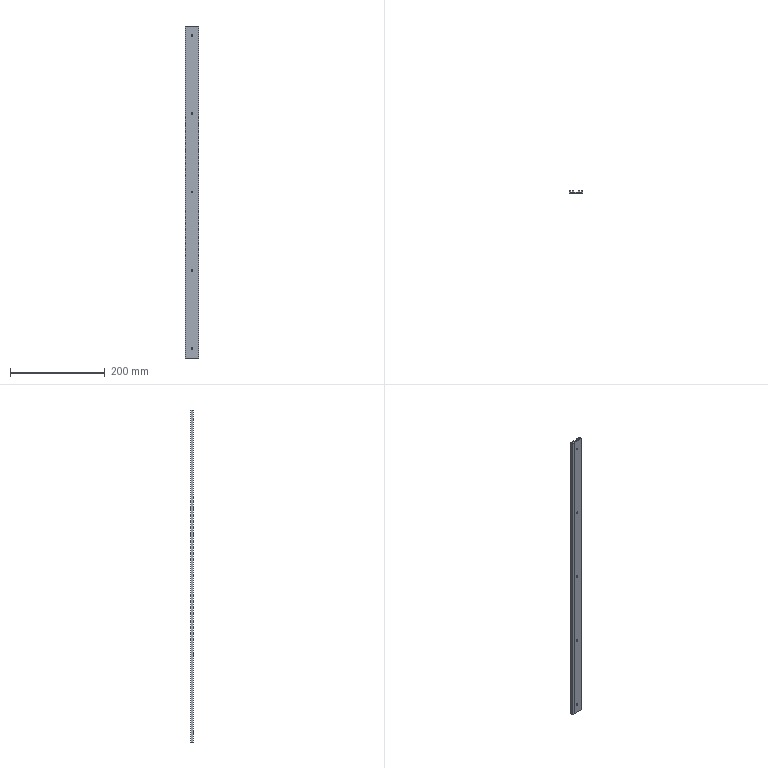Part | SolidWorks | features BaseBody 1, HoleWzd 1, ICE 1 | 1 solid | 36 faces | box 28 x 6 x 700 mm | volume 58418 mm3 | plane 26 | cylinder 10 | commonest cylinder face diameters 3.6 x10
STEP:
#1=CARTESIAN_POINT('',(0.,0.,-81.8));
#2=VERTEX_POINT('',#1);
#3=CARTESIAN_POINT('',(0.,0.,-78.2));
#4=VERTEX_POINT('',#3);
#5=CARTESIAN_POINT('',(0.,0.,-80.));
#6=DIRECTION('',(0.,1.,0.));
#7=DIRECTION('',(0.,0.,1.));
#8=AXIS2_PLACEMENT_3D('',#5,#6,#7);
#9=CIRCLE('',#8,1.8);
#10=EDGE_CURVE('',#2,#4,#9,.T.);
#11=ORIENTED_EDGE('',*,*,#10,.F.);
#12=CARTESIAN_POINT('',(0.,2.,-81.8));
#13=VERTEX_POINT('',#12);
#14=CARTESIAN_POINT('',(0.,2.,-81.8));
#15=DIRECTION('',(0.,1.,0.));
#16=VECTOR('',#15,1000.);
#17=LINE('',#14,#16);
#18=EDGE_CURVE('',#2,#13,#17,.T.);
#19=ORIENTED_EDGE('',*,*,#18,.T.);
#20=CARTESIAN_POINT('',(0.,2.,-78.2));
#21=VERTEX_POINT('',#20);
#22=CARTESIAN_POINT('',(0.,2.,-80.));
#23=DIRECTION('',(0.,1.,0.));
#24=DIRECTION('',(0.,0.,1.));
#25=AXIS2_PLACEMENT_3D('',#22,#23,#24);
#26=CIRCLE('',#25,1.8);
#27=EDGE_CURVE('',#13,#21,#26,.T.);
#28=ORIENTED_EDGE('',*,*,#27,.T.);
#29=CARTESIAN_POINT('',(0.,2.,-78.2));
#30=DIRECTION('',(0.,1.,0.));
#31=VECTOR('',#30,1000.);
#32=LINE('',#29,#31);
#33=EDGE_CURVE('',#4,#21,#32,.T.);
#34=ORIENTED_EDGE('',*,*,#33,.F.);
#35=EDGE_LOOP('',(#11,#19,#28,#34));
#36=FACE_OUTER_BOUND('',#35,.T.);
#37=CARTESIAN_POINT('',(0.,2.,-80.));
#38=DIRECTION('',(0.,1.,0.));
#39=DIRECTION('',(0.,0.,1.));
#40=AXIS2_PLACEMENT_3D('',#37,#38,#39);
#41=CYLINDRICAL_SURFACE('',#40,1.8);
#42=ADVANCED_FACE('',(#36),#41,.F.);
#43=CARTESIAN_POINT('',(0.,0.,83.2));
#44=VERTEX_POINT('',#43);
#45=CARTESIAN_POINT('',(0.,0.,86.8));
#46=VERTEX_POINT('',#45);
#47=CARTESIAN_POINT('',(0.,0.,85.));
#48=DIRECTION('',(0.,1.,0.));
#49=DIRECTION('',(0.,0.,1.));
#50=AXIS2_PLACEMENT_3D('',#47,#48,#49);
#51=CIRCLE('',#50,1.8);
#52=EDGE_CURVE('',#44,#46,#51,.T.);
#53=ORIENTED_EDGE('',*,*,#52,.F.);
#54=CARTESIAN_POINT('',(0.,2.,83.2));
#55=VERTEX_POINT('',#54);
#56=CARTESIAN_POINT('',(0.,2.,83.2));
#57=DIRECTION('',(0.,1.,0.));
#58=VECTOR('',#57,1000.);
#59=LINE('',#56,#58);
#60=EDGE_CURVE('',#44,#55,#59,.T.);
#61=ORIENTED_EDGE('',*,*,#60,.T.);
#62=CARTESIAN_POINT('',(0.,2.,86.8));
#63=VERTEX_POINT('',#62);
#64=CARTESIAN_POINT('',(0.,2.,85.));
#65=DIRECTION('',(0.,1.,0.));
#66=DIRECTION('',(0.,0.,1.));
#67=AXIS2_PLACEMENT_3D('',#64,#65,#66);
#68=CIRCLE('',#67,1.8);
#69=EDGE_CURVE('',#55,#63,#68,.T.);
#70=ORIENTED_EDGE('',*,*,#69,.T.);
#71=CARTESIAN_POINT('',(0.,2.,86.8));
#72=DIRECTION('',(0.,1.,0.));
#73=VECTOR('',#72,1000.);
#74=LINE('',#71,#73);
#75=EDGE_CURVE('',#46,#63,#74,.T.);
#76=ORIENTED_EDGE('',*,*,#75,.F.);
#77=EDGE_LOOP('',(#53,#61,#70,#76));
#78=FACE_OUTER_BOUND('',#77,.T.);
#79=CARTESIAN_POINT('',(0.,2.,85.));
#80=DIRECTION('',(0.,1.,0.));
#81=DIRECTION('',(0.,0.,1.));
#82=AXIS2_PLACEMENT_3D('',#79,#80,#81);
#83=CYLINDRICAL_SURFACE('',#82,1.8);
#84=ADVANCED_FACE('',(#78),#83,.F.);
#85=CARTESIAN_POINT('',(0.,0.,248.2));
#86=VERTEX_POINT('',#85);
#87=CARTESIAN_POINT('',(0.,0.,251.8));
#88=VERTEX_POINT('',#87);
#89=CARTESIAN_POINT('',(0.,0.,250.));
#90=DIRECTION('',(0.,1.,0.));
#91=DIRECTION('',(0.,0.,1.));
#92=AXIS2_PLACEMENT_3D('',#89,#90,#91);
#93=CIRCLE('',#92,1.8);
#94=EDGE_CURVE('',#86,#88,#93,.T.);
#95=ORIENTED_EDGE('',*,*,#94,.F.);
#96=CARTESIAN_POINT('',(0.,2.,248.2));
#97=VERTEX_POINT('',#96);
#98=CARTESIAN_POINT('',(0.,2.,248.2));
#99=DIRECTION('',(0.,1.,0.));
#100=VECTOR('',#99,1000.);
#101=LINE('',#98,#100);
#102=EDGE_CURVE('',#86,#97,#101,.T.);
#103=ORIENTED_EDGE('',*,*,#102,.T.);
#104=CARTESIAN_POINT('',(0.,2.,251.8));
#105=VERTEX_POINT('',#104);
#106=CARTESIAN_POINT('',(0.,2.,250.));
#107=DIRECTION('',(0.,1.,0.));
#108=DIRECTION('',(0.,0.,1.));
#109=AXIS2_PLACEMENT_3D('',#106,#107,#108);
#110=CIRCLE('',#109,1.8);
#111=EDGE_CURVE('',#97,#105,#110,.T.);
#112=ORIENTED_EDGE('',*,*,#111,.T.);
#113=CARTESIAN_POINT('',(0.,2.,251.8));
#114=DIRECTION('',(0.,1.,0.));
#115=VECTOR('',#114,1000.);
#116=LINE('',#113,#115);
#117=EDGE_CURVE('',#88,#105,#116,.T.);
#118=ORIENTED_EDGE('',*,*,#117,.F.);
#119=EDGE_LOOP('',(#95,#103,#112,#118));
#120=FACE_OUTER_BOUND('',#119,.T.);
#121=CARTESIAN_POINT('',(0.,2.,250.));
#122=DIRECTION('',(0.,1.,0.));
#123=DIRECTION('',(0.,0.,1.));
#124=AXIS2_PLACEMENT_3D('',#121,#122,#123);
#125=CYLINDRICAL_SURFACE('',#124,1.8);
#126=ADVANCED_FACE('',(#120),#125,.F.);
#127=CARTESIAN_POINT('',(0.,0.,413.2));
#128=VERTEX_POINT('',#127);
#129=CARTESIAN_POINT('',(0.,0.,416.8));
#130=VERTEX_POINT('',#129);
#131=CARTESIAN_POINT('',(0.,0.,415.));
#132=DIRECTION('',(0.,1.,0.));
#133=DIRECTION('',(0.,0.,1.));
#134=AXIS2_PLACEMENT_3D('',#131,#132,#133);
#135=CIRCLE('',#134,1.8);
#136=EDGE_CURVE('',#128,#130,#135,.T.);
#137=ORIENTED_EDGE('',*,*,#136,.F.);
#138=CARTESIAN_POINT('',(0.,2.,413.2));
#139=VERTEX_POINT('',#138);
#140=CARTESIAN_POINT('',(0.,2.,413.2));
#141=DIRECTION('',(0.,1.,0.));
#142=VECTOR('',#141,1000.);
#143=LINE('',#140,#142);
#144=EDGE_CURVE('',#128,#139,#143,.T.);
#145=ORIENTED_EDGE('',*,*,#144,.T.);
#146=CARTESIAN_POINT('',(0.,2.,416.8));
#147=VERTEX_POINT('',#146);
#148=CARTESIAN_POINT('',(0.,2.,415.));
#149=DIRECTION('',(0.,1.,0.));
#150=DIRECTION('',(0.,0.,1.));
#151=AXIS2_PLACEMENT_3D('',#148,#149,#150);
#152=CIRCLE('',#151,1.8);
#153=EDGE_CURVE('',#139,#147,#152,.T.);
#154=ORIENTED_EDGE('',*,*,#153,.T.);
#155=CARTESIAN_POINT('',(0.,2.,416.8));
#156=DIRECTION('',(0.,1.,0.));
#157=VECTOR('',#156,1000.);
#158=LINE('',#155,#157);
#159=EDGE_CURVE('',#130,#147,#158,.T.);
#160=ORIENTED_EDGE('',*,*,#159,.F.);
#161=EDGE_LOOP('',(#137,#145,#154,#160));
#162=FACE_OUTER_BOUND('',#161,.T.);
#163=CARTESIAN_POINT('',(0.,2.,415.));
#164=DIRECTION('',(0.,1.,0.));
#165=DIRECTION('',(0.,0.,1.));
#166=AXIS2_PLACEMENT_3D('',#163,#164,#165);
#167=CYLINDRICAL_SURFACE('',#166,1.8);
#168=ADVANCED_FACE('',(#162),#167,.F.);
#169=CARTESIAN_POINT('',(0.,0.,578.2));
#170=VERTEX_POINT('',#169);
#171=CARTESIAN_POINT('',(0.,0.,581.8));
#172=VERTEX_POINT('',#171);
#173=CARTESIAN_POINT('',(0.,0.,580.));
#174=DIRECTION('',(0.,1.,0.));
#175=DIRECTION('',(0.,0.,1.));
#176=AXIS2_PLACEMENT_3D('',#173,#174,#175);
#177=CIRCLE('',#176,1.8);
#178=EDGE_CURVE('',#170,#172,#177,.T.);
#179=ORIENTED_EDGE('',*,*,#178,.F.);
#180=CARTESIAN_POINT('',(0.,2.,578.2));
#181=VERTEX_POINT('',#180);
#182=CARTESIAN_POINT('',(0.,2.,578.2));
#183=DIRECTION('',(0.,1.,0.));
#184=VECTOR('',#183,1000.);
#185=LINE('',#182,#184);
#186=EDGE_CURVE('',#170,#181,#185,.T.);
#187=ORIENTED_EDGE('',*,*,#186,.T.);
#188=CARTESIAN_POINT('',(0.,2.,581.8));
#189=VERTEX_POINT('',#188);
#190=CARTESIAN_POINT('',(0.,2.,580.));
#191=DIRECTION('',(0.,1.,0.));
#192=DIRECTION('',(0.,0.,1.));
#193=AXIS2_PLACEMENT_3D('',#190,#191,#192);
#194=CIRCLE('',#193,1.8);
#195=EDGE_CURVE('',#181,#189,#194,.T.);
#196=ORIENTED_EDGE('',*,*,#195,.T.);
#197=CARTESIAN_POINT('',(0.,2.,581.8));
#198=DIRECTION('',(0.,1.,0.));
#199=VECTOR('',#198,1000.);
#200=LINE('',#197,#199);
#201=EDGE_CURVE('',#172,#189,#200,.T.);
#202=ORIENTED_EDGE('',*,*,#201,.F.);
#203=EDGE_LOOP('',(#179,#187,#196,#202));
#204=FACE_OUTER_BOUND('',#203,.T.);
#205=CARTESIAN_POINT('',(0.,2.,580.));
#206=DIRECTION('',(0.,1.,0.));
#207=DIRECTION('',(0.,0.,1.));
#208=AXIS2_PLACEMENT_3D('',#205,#206,#207);
#209=CYLINDRICAL_SURFACE('',#208,1.8);
#210=ADVANCED_FACE('',(#204),#209,.F.);
#211=CARTESIAN_POINT('',(0.,0.,-80.));
#212=DIRECTION('',(0.,1.,0.));
#213=DIRECTION('',(0.,0.,1.));
#214=AXIS2_PLACEMENT_3D('',#211,#212,#213);
#215=CIRCLE('',#214,1.8);
#216=EDGE_CURVE('',#4,#2,#215,.T.);
#217=ORIENTED_EDGE('',*,*,#216,.T.);
#218=ORIENTED_EDGE('',*,*,#10,.T.);
#219=EDGE_LOOP('',(#217,#218));
#220=FACE_BOUND('',#219,.T.);
#221=CARTESIAN_POINT('',(0.,0.,85.));
#222=DIRECTION('',(0.,1.,0.));
#223=DIRECTION('',(0.,0.,1.));
#224=AXIS2_PLACEMENT_3D('',#221,#222,#223);
#225=CIRCLE('',#224,1.8);
#226=EDGE_CURVE('',#46,#44,#225,.T.);
#227=ORIENTED_EDGE('',*,*,#226,.T.);
#228=ORIENTED_EDGE('',*,*,#52,.T.);
#229=EDGE_LOOP('',(#227,#228));
#230=FACE_BOUND('',#229,.T.);
#231=CARTESIAN_POINT('',(0.,0.,250.));
#232=DIRECTION('',(0.,1.,0.));
#233=DIRECTION('',(0.,0.,1.));
#234=AXIS2_PLACEMENT_3D('',#231,#232,#233);
#235=CIRCLE('',#234,1.8);
#236=EDGE_CURVE('',#88,#86,#235,.T.);
#237=ORIENTED_EDGE('',*,*,#236,.T.);
#238=ORIENTED_EDGE('',*,*,#94,.T.);
#239=EDGE_LOOP('',(#237,#238));
#240=FACE_BOUND('',#239,.T.);
#241=CARTESIAN_POINT('',(0.,0.,415.));
#242=DIRECTION('',(0.,1.,0.));
#243=DIRECTION('',(0.,0.,1.));
#244=AXIS2_PLACEMENT_3D('',#241,#242,#243);
#245=CIRCLE('',#244,1.8);
#246=EDGE_CURVE('',#130,#128,#245,.T.);
#247=ORIENTED_EDGE('',*,*,#246,.T.);
#248=ORIENTED_EDGE('',*,*,#136,.T.);
#249=EDGE_LOOP('',(#247,#248));
#250=FACE_BOUND('',#249,.T.);
#251=CARTESIAN_POINT('',(0.,0.,580.));
#252=DIRECTION('',(0.,1.,0.));
#253=DIRECTION('',(0.,0.,1.));
#254=AXIS2_PLACEMENT_3D('',#251,#252,#253);
#255=CIRCLE('',#254,1.8);
#256=EDGE_CURVE('',#172,#170,#255,.T.);
#257=ORIENTED_EDGE('',*,*,#256,.T.);
#258=ORIENTED_EDGE('',*,*,#178,.T.);
#259=EDGE_LOOP('',(#257,#258));
#260=FACE_BOUND('',#259,.T.);
#261=CARTESIAN_POINT('',(-14.,0.,-100.));
#262=VERTEX_POINT('',#261);
#263=CARTESIAN_POINT('',(14.,0.,-100.));
#264=VERTEX_POINT('',#263);
#265=CARTESIAN_POINT('',(-14.,0.,-100.));
#266=DIRECTION('',(1.,0.,0.));
#267=VECTOR('',#266,1000.);
#268=LINE('',#265,#267);
#269=EDGE_CURVE('',#262,#264,#268,.T.);
#270=ORIENTED_EDGE('',*,*,#269,.T.);
#271=CARTESIAN_POINT('',(14.,0.,600.));
#272=VERTEX_POINT('',#271);
#273=CARTESIAN_POINT('',(14.,0.,-100.));
#274=DIRECTION('',(0.,0.,1.));
#275=VECTOR('',#274,1000.);
#276=LINE('',#273,#275);
#277=EDGE_CURVE('',#264,#272,#276,.T.);
#278=ORIENTED_EDGE('',*,*,#277,.T.);
#279=CARTESIAN_POINT('',(-14.,0.,600.));
#280=VERTEX_POINT('',#279);
#281=CARTESIAN_POINT('',(-14.,0.,600.));
#282=DIRECTION('',(1.,0.,0.));
#283=VECTOR('',#282,1000.);
#284=LINE('',#281,#283);
#285=EDGE_CURVE('',#280,#272,#284,.T.);
#286=ORIENTED_EDGE('',*,*,#285,.F.);
#287=CARTESIAN_POINT('',(-14.,0.,-100.));
#288=DIRECTION('',(0.,0.,-1.));
#289=VECTOR('',#288,1000.);
#290=LINE('',#287,#289);
#291=EDGE_CURVE('',#280,#262,#290,.T.);
#292=ORIENTED_EDGE('',*,*,#291,.T.);
#293=EDGE_LOOP('',(#270,#278,#286,#292));
#294=FACE_OUTER_BOUND('',#293,.T.);
#295=CARTESIAN_POINT('',(-14.,0.,-100.));
#296=DIRECTION('',(0.,-1.,0.));
#297=DIRECTION('',(0.,0.,-1.));
#298=AXIS2_PLACEMENT_3D('',#295,#296,#297);
#299=PLANE('',#298);
#300=ADVANCED_FACE('',(#220,#230,#240,#250,#260,#294),#299,.T.);
#301=CARTESIAN_POINT('',(14.,6.,-100.));
#302=VERTEX_POINT('',#301);
#303=CARTESIAN_POINT('',(14.,0.,-100.));
#304=DIRECTION('',(0.,1.,0.));
#305=VECTOR('',#304,1000.);
#306=LINE('',#303,#305);
#307=EDGE_CURVE('',#264,#302,#306,.T.);
#308=ORIENTED_EDGE('',*,*,#307,.T.);
#309=CARTESIAN_POINT('',(14.,6.,600.));
#310=VERTEX_POINT('',#309);
#311=CARTESIAN_POINT('',(14.,6.,-100.));
#312=DIRECTION('',(0.,0.,1.));
#313=VECTOR('',#312,1000.);
#314=LINE('',#311,#313);
#315=EDGE_CURVE('',#302,#310,#314,.T.);
#316=ORIENTED_EDGE('',*,*,#315,.T.);
#317=CARTESIAN_POINT('',(14.,0.,600.));
#318=DIRECTION('',(0.,1.,0.));
#319=VECTOR('',#318,1000.);
#320=LINE('',#317,#319);
#321=EDGE_CURVE('',#272,#310,#320,.T.);
#322=ORIENTED_EDGE('',*,*,#321,.F.);
#323=ORIENTED_EDGE('',*,*,#277,.F.);
#324=EDGE_LOOP('',(#308,#316,#322,#323));
#325=FACE_OUTER_BOUND('',#324,.T.);
#326=CARTESIAN_POINT('',(14.,0.,-100.));
#327=DIRECTION('',(1.,0.,0.));
#328=DIRECTION('',(0.,0.,-1.));
#329=AXIS2_PLACEMENT_3D('',#326,#327,#328);
#330=PLANE('',#329);
#331=ADVANCED_FACE('',(#325),#330,.T.);
#332=CARTESIAN_POINT('',(-11.2,6.,-100.));
#333=VERTEX_POINT('',#332);
#334=CARTESIAN_POINT('',(-14.,6.,-100.));
#335=VERTEX_POINT('',#334);
#336=CARTESIAN_POINT('',(0.,6.,-100.));
#337=DIRECTION('',(-1.,0.,0.));
#338=VECTOR('',#337,1000.);
#339=LINE('',#336,#338);
#340=EDGE_CURVE('',#333,#335,#339,.T.);
#341=ORIENTED_EDGE('',*,*,#340,.F.);
#342=CARTESIAN_POINT('',(-11.2,4.5,-100.));
#343=VERTEX_POINT('',#342);
#344=CARTESIAN_POINT('',(-11.2,4.5,-100.));
#345=DIRECTION('',(0.,1.,0.));
#346=VECTOR('',#345,1000.);
#347=LINE('',#344,#346);
#348=EDGE_CURVE('',#343,#333,#347,.T.);
#349=ORIENTED_EDGE('',*,*,#348,.F.);
#350=CARTESIAN_POINT('',(-12.35,4.5,-100.));
#351=VERTEX_POINT('',#350);
#352=CARTESIAN_POINT('',(-12.35,4.5,-100.));
#353=DIRECTION('',(1.,0.,0.));
#354=VECTOR('',#353,1000.);
#355=LINE('',#352,#354);
#356=EDGE_CURVE('',#351,#343,#355,.T.);
#357=ORIENTED_EDGE('',*,*,#356,.F.);
#358=CARTESIAN_POINT('',(-12.35,1.5,-100.));
#359=VERTEX_POINT('',#358);
#360=CARTESIAN_POINT('',(-12.35,0.,-100.));
#361=DIRECTION('',(0.,1.,0.));
#362=VECTOR('',#361,1000.);
#363=LINE('',#360,#362);
#364=EDGE_CURVE('',#359,#351,#363,.T.);
#365=ORIENTED_EDGE('',*,*,#364,.F.);
#366=CARTESIAN_POINT('',(-6.65,1.5,-100.));
#367=VERTEX_POINT('',#366);
#368=CARTESIAN_POINT('',(0.,1.5,-100.));
#369=DIRECTION('',(-1.,0.,0.));
#370=VECTOR('',#369,1000.);
#371=LINE('',#368,#370);
#372=EDGE_CURVE('',#367,#359,#371,.T.);
#373=ORIENTED_EDGE('',*,*,#372,.F.);
#374=CARTESIAN_POINT('',(-6.65,4.5,-100.));
#375=VERTEX_POINT('',#374);
#376=CARTESIAN_POINT('',(-6.65,0.,-100.));
#377=DIRECTION('',(0.,-1.,0.));
#378=VECTOR('',#377,1000.);
#379=LINE('',#376,#378);
#380=EDGE_CURVE('',#375,#367,#379,.T.);
#381=ORIENTED_EDGE('',*,*,#380,.F.);
#382=CARTESIAN_POINT('',(-7.8,4.5,-100.));
#383=VERTEX_POINT('',#382);
#384=CARTESIAN_POINT('',(-7.8,4.5,-100.));
#385=DIRECTION('',(1.,0.,0.));
#386=VECTOR('',#385,1000.);
#387=LINE('',#384,#386);
#388=EDGE_CURVE('',#383,#375,#387,.T.);
#389=ORIENTED_EDGE('',*,*,#388,.F.);
#390=CARTESIAN_POINT('',(-7.8,6.,-100.));
#391=VERTEX_POINT('',#390);
#392=CARTESIAN_POINT('',(-7.8,6.,-100.));
#393=DIRECTION('',(0.,-1.,0.));
#394=VECTOR('',#393,1000.);
#395=LINE('',#392,#394);
#396=EDGE_CURVE('',#391,#383,#395,.T.);
#397=ORIENTED_EDGE('',*,*,#396,.F.);
#398=CARTESIAN_POINT('',(-5.,6.,-100.));
#399=VERTEX_POINT('',#398);
#400=CARTESIAN_POINT('',(0.,6.,-100.));
#401=DIRECTION('',(-1.,0.,0.));
#402=VECTOR('',#401,1000.);
#403=LINE('',#400,#402);
#404=EDGE_CURVE('',#399,#391,#403,.T.);
#405=ORIENTED_EDGE('',*,*,#404,.F.);
#406=CARTESIAN_POINT('',(-5.,2.,-100.));
#407=VERTEX_POINT('',#406);
#408=CARTESIAN_POINT('',(-5.,0.,-100.));
#409=DIRECTION('',(0.,1.,0.));
#410=VECTOR('',#409,1000.);
#411=LINE('',#408,#410);
#412=EDGE_CURVE('',#407,#399,#411,.T.);
#413=ORIENTED_EDGE('',*,*,#412,.F.);
#414=CARTESIAN_POINT('',(5.,2.,-100.));
#415=VERTEX_POINT('',#414);
#416=CARTESIAN_POINT('',(0.,2.,-100.));
#417=DIRECTION('',(-1.,0.,0.));
#418=VECTOR('',#417,1000.);
#419=LINE('',#416,#418);
#420=EDGE_CURVE('',#415,#407,#419,.T.);
#421=ORIENTED_EDGE('',*,*,#420,.F.);
#422=CARTESIAN_POINT('',(5.,6.,-100.));
#423=VERTEX_POINT('',#422);
#424=CARTESIAN_POINT('',(5.,0.,-100.));
#425=DIRECTION('',(0.,-1.,0.));
#426=VECTOR('',#425,1000.);
#427=LINE('',#424,#426);
#428=EDGE_CURVE('',#423,#415,#427,.T.);
#429=ORIENTED_EDGE('',*,*,#428,.F.);
#430=CARTESIAN_POINT('',(7.8,6.,-100.));
#431=VERTEX_POINT('',#430);
#432=CARTESIAN_POINT('',(0.,6.,-100.));
#433=DIRECTION('',(-1.,0.,0.));
#434=VECTOR('',#433,1000.);
#435=LINE('',#432,#434);
#436=EDGE_CURVE('',#431,#423,#435,.T.);
#437=ORIENTED_EDGE('',*,*,#436,.F.);
#438=CARTESIAN_POINT('',(7.8,4.5,-100.));
#439=VERTEX_POINT('',#438);
#440=CARTESIAN_POINT('',(7.8,4.5,-100.));
#441=DIRECTION('',(0.,1.,0.));
#442=VECTOR('',#441,1000.);
#443=LINE('',#440,#442);
#444=EDGE_CURVE('',#439,#431,#443,.T.);
#445=ORIENTED_EDGE('',*,*,#444,.F.);
#446=CARTESIAN_POINT('',(6.65,4.5,-100.));
#447=VERTEX_POINT('',#446);
#448=CARTESIAN_POINT('',(6.65,4.5,-100.));
#449=DIRECTION('',(1.,0.,0.));
#450=VECTOR('',#449,1000.);
#451=LINE('',#448,#450);
#452=EDGE_CURVE('',#447,#439,#451,.T.);
#453=ORIENTED_EDGE('',*,*,#452,.F.);
#454=CARTESIAN_POINT('',(6.65,1.5,-100.));
#455=VERTEX_POINT('',#454);
#456=CARTESIAN_POINT('',(6.65,0.,-100.));
#457=DIRECTION('',(0.,1.,0.));
#458=VECTOR('',#457,1000.);
#459=LINE('',#456,#458);
#460=EDGE_CURVE('',#455,#447,#459,.T.);
#461=ORIENTED_EDGE('',*,*,#460,.F.);
#462=CARTESIAN_POINT('',(12.35,1.5,-100.));
#463=VERTEX_POINT('',#462);
#464=CARTESIAN_POINT('',(0.,1.5,-100.));
#465=DIRECTION('',(-1.,0.,0.));
#466=VECTOR('',#465,1000.);
#467=LINE('',#464,#466);
#468=EDGE_CURVE('',#463,#455,#467,.T.);
#469=ORIENTED_EDGE('',*,*,#468,.F.);
#470=CARTESIAN_POINT('',(12.35,4.5,-100.));
#471=VERTEX_POINT('',#470);
#472=CARTESIAN_POINT('',(12.35,0.,-100.));
#473=DIRECTION('',(0.,-1.,0.));
#474=VECTOR('',#473,1000.);
#475=LINE('',#472,#474);
#476=EDGE_CURVE('',#471,#463,#475,.T.);
#477=ORIENTED_EDGE('',*,*,#476,.F.);
#478=CARTESIAN_POINT('',(11.2,4.5,-100.));
#479=VERTEX_POINT('',#478);
#480=CARTESIAN_POINT('',(11.2,4.5,-100.));
#481=DIRECTION('',(1.,0.,0.));
#482=VECTOR('',#481,1000.);
#483=LINE('',#480,#482);
#484=EDGE_CURVE('',#479,#471,#483,.T.);
#485=ORIENTED_EDGE('',*,*,#484,.F.);
#486=CARTESIAN_POINT('',(11.2,6.,-100.));
#487=VERTEX_POINT('',#486);
#488=CARTESIAN_POINT('',(11.2,6.,-100.));
#489=DIRECTION('',(0.,-1.,0.));
#490=VECTOR('',#489,1000.);
#491=LINE('',#488,#490);
#492=EDGE_CURVE('',#487,#479,#491,.T.);
#493=ORIENTED_EDGE('',*,*,#492,.F.);
#494=CARTESIAN_POINT('',(0.,6.,-100.));
#495=DIRECTION('',(-1.,0.,0.));
#496=VECTOR('',#495,1000.);
#497=LINE('',#494,#496);
#498=EDGE_CURVE('',#302,#487,#497,.T.);
#499=ORIENTED_EDGE('',*,*,#498,.F.);
#500=ORIENTED_EDGE('',*,*,#307,.F.);
#501=ORIENTED_EDGE('',*,*,#269,.F.);
#502=CARTESIAN_POINT('',(-14.,0.,-100.));
#503=DIRECTION('',(0.,-1.,0.));
#504=VECTOR('',#503,1000.);
#505=LINE('',#502,#504);
#506=EDGE_CURVE('',#335,#262,#505,.T.);
#507=ORIENTED_EDGE('',*,*,#506,.F.);
#508=EDGE_LOOP('',(#341,#349,#357,#365,#373,#381,#389,#397,#405,#413,#421,#429,#437,#445,#453,#461,#469,#477,#485,#493,#499,#500,#501,#507));
#509=FACE_OUTER_BOUND('',#508,.T.);
#510=CARTESIAN_POINT('',(0.,0.,-100.));
#511=DIRECTION('',(0.,0.,1.));
#512=DIRECTION('',(1.,0.,0.));
#513=AXIS2_PLACEMENT_3D('',#510,#511,#512);
#514=PLANE('',#513);
#515=ADVANCED_FACE('',(#509),#514,.F.);
#516=ORIENTED_EDGE('',*,*,#506,.T.);
#517=ORIENTED_EDGE('',*,*,#291,.F.);
#518=CARTESIAN_POINT('',(-14.,6.,600.));
#519=VERTEX_POINT('',#518);
#520=CARTESIAN_POINT('',(-14.,6.,600.));
#521=DIRECTION('',(0.,-1.,0.));
#522=VECTOR('',#521,1000.);
#523=LINE('',#520,#522);
#524=EDGE_CURVE('',#519,#280,#523,.T.);
#525=ORIENTED_EDGE('',*,*,#524,.F.);
#526=CARTESIAN_POINT('',(-14.,6.,-100.));
#527=DIRECTION('',(0.,0.,-1.));
#528=VECTOR('',#527,1000.);
#529=LINE('',#526,#528);
#530=EDGE_CURVE('',#519,#335,#529,.T.);
#531=ORIENTED_EDGE('',*,*,#530,.T.);
#532=EDGE_LOOP('',(#516,#517,#525,#531));
#533=FACE_OUTER_BOUND('',#532,.T.);
#534=CARTESIAN_POINT('',(-14.,6.,-100.));
#535=DIRECTION('',(-1.,0.,0.));
#536=DIRECTION('',(0.,0.,1.));
#537=AXIS2_PLACEMENT_3D('',#534,#535,#536);
#538=PLANE('',#537);
#539=ADVANCED_FACE('',(#533),#538,.T.);
#540=ORIENTED_EDGE('',*,*,#498,.T.);
#541=CARTESIAN_POINT('',(11.2,6.,600.));
#542=VERTEX_POINT('',#541);
#543=CARTESIAN_POINT('',(11.2,6.,-100.));
#544=DIRECTION('',(0.,0.,1.));
#545=VECTOR('',#544,1000.);
#546=LINE('',#543,#545);
#547=EDGE_CURVE('',#487,#542,#546,.T.);
#548=ORIENTED_EDGE('',*,*,#547,.T.);
#549=CARTESIAN_POINT('',(14.,6.,600.));
#550=DIRECTION('',(-1.,0.,0.));
#551=VECTOR('',#550,1000.);
#552=LINE('',#549,#551);
#553=EDGE_CURVE('',#310,#542,#552,.T.);
#554=ORIENTED_EDGE('',*,*,#553,.F.);
#555=ORIENTED_EDGE('',*,*,#315,.F.);
#556=EDGE_LOOP('',(#540,#548,#554,#555));
#557=FACE_OUTER_BOUND('',#556,.T.);
#558=CARTESIAN_POINT('',(14.,6.,-100.));
#559=DIRECTION('',(0.,1.,0.));
#560=DIRECTION('',(0.,0.,1.));
#561=AXIS2_PLACEMENT_3D('',#558,#559,#560);
#562=PLANE('',#561);
#563=ADVANCED_FACE('',(#557),#562,.T.);
#564=ORIENTED_EDGE('',*,*,#340,.T.);
#565=ORIENTED_EDGE('',*,*,#530,.F.);
#566=CARTESIAN_POINT('',(-11.2,6.,600.));
#567=VERTEX_POINT('',#566);
#568=CARTESIAN_POINT('',(-11.2,6.,600.));
#569=DIRECTION('',(-1.,0.,0.));
#570=VECTOR('',#569,1000.);
#571=LINE('',#568,#570);
#572=EDGE_CURVE('',#567,#519,#571,.T.);
#573=ORIENTED_EDGE('',*,*,#572,.F.);
#574=CARTESIAN_POINT('',(-11.2,6.,-100.));
#575=DIRECTION('',(0.,0.,-1.));
#576=VECTOR('',#575,1000.);
#577=LINE('',#574,#576);
#578=EDGE_CURVE('',#567,#333,#577,.T.);
#579=ORIENTED_EDGE('',*,*,#578,.T.);
#580=EDGE_LOOP('',(#564,#565,#573,#579));
#581=FACE_OUTER_BOUND('',#580,.T.);
#582=CARTESIAN_POINT('',(-11.2,6.,-100.));
#583=DIRECTION('',(0.,1.,0.));
#584=DIRECTION('',(0.,0.,1.));
#585=AXIS2_PLACEMENT_3D('',#582,#583,#584);
#586=PLANE('',#585);
#587=ADVANCED_FACE('',(#581),#586,.T.);
#588=ORIENTED_EDGE('',*,*,#364,.T.);
#589=CARTESIAN_POINT('',(-12.35,4.5,600.));
#590=VERTEX_POINT('',#589);
#591=CARTESIAN_POINT('',(-12.35,4.5,-100.));
#592=DIRECTION('',(0.,0.,1.));
#593=VECTOR('',#592,1000.);
#594=LINE('',#591,#593);
#595=EDGE_CURVE('',#351,#590,#594,.T.);
#596=ORIENTED_EDGE('',*,*,#595,.T.);
#597=CARTESIAN_POINT('',(-12.35,1.5,600.));
#598=VERTEX_POINT('',#597);
#599=CARTESIAN_POINT('',(-12.35,1.5,600.));
#600=DIRECTION('',(0.,1.,0.));
#601=VECTOR('',#600,1000.);
#602=LINE('',#599,#601);
#603=EDGE_CURVE('',#598,#590,#602,.T.);
#604=ORIENTED_EDGE('',*,*,#603,.F.);
#605=CARTESIAN_POINT('',(-12.35,1.5,-100.));
#606=DIRECTION('',(0.,0.,-1.));
#607=VECTOR('',#606,1000.);
#608=LINE('',#605,#607);
#609=EDGE_CURVE('',#598,#359,#608,.T.);
#610=ORIENTED_EDGE('',*,*,#609,.T.);
#611=EDGE_LOOP('',(#588,#596,#604,#610));
#612=FACE_OUTER_BOUND('',#611,.T.);
#613=CARTESIAN_POINT('',(-12.35,1.5,-100.));
#614=DIRECTION('',(1.,0.,0.));
#615=DIRECTION('',(0.,0.,-1.));
#616=AXIS2_PLACEMENT_3D('',#613,#614,#615);
#617=PLANE('',#616);
#618=ADVANCED_FACE('',(#612),#617,.T.);
#619=ORIENTED_EDGE('',*,*,#372,.T.);
#620=ORIENTED_EDGE('',*,*,#609,.F.);
#621=CARTESIAN_POINT('',(-6.65,1.5,600.));
#622=VERTEX_POINT('',#621);
#623=CARTESIAN_POINT('',(-6.65,1.5,600.));
#624=DIRECTION('',(-1.,0.,0.));
#625=VECTOR('',#624,1000.);
#626=LINE('',#623,#625);
#627=EDGE_CURVE('',#622,#598,#626,.T.);
#628=ORIENTED_EDGE('',*,*,#627,.F.);
#629=CARTESIAN_POINT('',(-6.65,1.5,-100.));
#630=DIRECTION('',(0.,0.,-1.));
#631=VECTOR('',#630,1000.);
#632=LINE('',#629,#631);
#633=EDGE_CURVE('',#622,#367,#632,.T.);
#634=ORIENTED_EDGE('',*,*,#633,.T.);
#635=EDGE_LOOP('',(#619,#620,#628,#634));
#636=FACE_OUTER_BOUND('',#635,.T.);
#637=CARTESIAN_POINT('',(-6.65,1.5,-100.));
#638=DIRECTION('',(0.,1.,0.));
#639=DIRECTION('',(0.,0.,1.));
#640=AXIS2_PLACEMENT_3D('',#637,#638,#639);
#641=PLANE('',#640);
#642=ADVANCED_FACE('',(#636),#641,.T.);
#643=ORIENTED_EDGE('',*,*,#380,.T.);
#644=ORIENTED_EDGE('',*,*,#633,.F.);
#645=CARTESIAN_POINT('',(-6.65,4.5,600.));
#646=VERTEX_POINT('',#645);
#647=CARTESIAN_POINT('',(-6.65,4.5,600.));
#648=DIRECTION('',(0.,-1.,0.));
#649=VECTOR('',#648,1000.);
#650=LINE('',#647,#649);
#651=EDGE_CURVE('',#646,#622,#650,.T.);
#652=ORIENTED_EDGE('',*,*,#651,.F.);
#653=CARTESIAN_POINT('',(-6.65,4.5,-100.));
#654=DIRECTION('',(0.,0.,-1.));
#655=VECTOR('',#654,1000.);
#656=LINE('',#653,#655);
#657=EDGE_CURVE('',#646,#375,#656,.T.);
#658=ORIENTED_EDGE('',*,*,#657,.T.);
#659=EDGE_LOOP('',(#643,#644,#652,#658));
#660=FACE_OUTER_BOUND('',#659,.T.);
#661=CARTESIAN_POINT('',(-6.65,4.5,-100.));
#662=DIRECTION('',(-1.,0.,0.));
#663=DIRECTION('',(0.,0.,1.));
#664=AXIS2_PLACEMENT_3D('',#661,#662,#663);
#665=PLANE('',#664);
#666=ADVANCED_FACE('',(#660),#665,.T.);
#667=ORIENTED_EDGE('',*,*,#404,.T.);
#668=CARTESIAN_POINT('',(-7.8,6.,600.));
#669=VERTEX_POINT('',#668);
#670=CARTESIAN_POINT('',(-7.8,6.,-100.));
#671=DIRECTION('',(0.,0.,1.));
#672=VECTOR('',#671,1000.);
#673=LINE('',#670,#672);
#674=EDGE_CURVE('',#391,#669,#673,.T.);
#675=ORIENTED_EDGE('',*,*,#674,.T.);
#676=CARTESIAN_POINT('',(-5.,6.,600.));
#677=VERTEX_POINT('',#676);
#678=CARTESIAN_POINT('',(-5.,6.,600.));
#679=DIRECTION('',(-1.,0.,0.));
#680=VECTOR('',#679,1000.);
#681=LINE('',#678,#680);
#682=EDGE_CURVE('',#677,#669,#681,.T.);
#683=ORIENTED_EDGE('',*,*,#682,.F.);
#684=CARTESIAN_POINT('',(-5.,6.,-100.));
#685=DIRECTION('',(0.,0.,-1.));
#686=VECTOR('',#685,1000.);
#687=LINE('',#684,#686);
#688=EDGE_CURVE('',#677,#399,#687,.T.);
#689=ORIENTED_EDGE('',*,*,#688,.T.);
#690=EDGE_LOOP('',(#667,#675,#683,#689));
#691=FACE_OUTER_BOUND('',#690,.T.);
#692=CARTESIAN_POINT('',(-5.,6.,-100.));
#693=DIRECTION('',(0.,1.,0.));
#694=DIRECTION('',(0.,0.,1.));
#695=AXIS2_PLACEMENT_3D('',#692,#693,#694);
#696=PLANE('',#695);
#697=ADVANCED_FACE('',(#691),#696,.T.);
#698=ORIENTED_EDGE('',*,*,#412,.T.);
#699=ORIENTED_EDGE('',*,*,#688,.F.);
#700=CARTESIAN_POINT('',(-5.,2.,600.));
#701=VERTEX_POINT('',#700);
#702=CARTESIAN_POINT('',(-5.,2.,600.));
#703=DIRECTION('',(0.,1.,0.));
#704=VECTOR('',#703,1000.);
#705=LINE('',#702,#704);
#706=EDGE_CURVE('',#701,#677,#705,.T.);
#707=ORIENTED_EDGE('',*,*,#706,.F.);
#708=CARTESIAN_POINT('',(-5.,2.,-100.));
#709=DIRECTION('',(0.,0.,-1.));
#710=VECTOR('',#709,1000.);
#711=LINE('',#708,#710);
#712=EDGE_CURVE('',#701,#407,#711,.T.);
#713=ORIENTED_EDGE('',*,*,#712,.T.);
#714=EDGE_LOOP('',(#698,#699,#707,#713));
#715=FACE_OUTER_BOUND('',#714,.T.);
#716=CARTESIAN_POINT('',(-5.,2.,-100.));
#717=DIRECTION('',(1.,0.,0.));
#718=DIRECTION('',(0.,0.,-1.));
#719=AXIS2_PLACEMENT_3D('',#716,#717,#718);
#720=PLANE('',#719);
#721=ADVANCED_FACE('',(#715),#720,.T.);
#722=CARTESIAN_POINT('',(0.,2.,-80.));
#723=DIRECTION('',(0.,1.,0.));
#724=DIRECTION('',(0.,0.,1.));
#725=AXIS2_PLACEMENT_3D('',#722,#723,#724);
#726=CIRCLE('',#725,1.8);
#727=EDGE_CURVE('',#21,#13,#726,.T.);
#728=ORIENTED_EDGE('',*,*,#727,.F.);
#729=ORIENTED_EDGE('',*,*,#27,.F.);
#730=EDGE_LOOP('',(#728,#729));
#731=FACE_BOUND('',#730,.T.);
#732=CARTESIAN_POINT('',(0.,2.,85.));
#733=DIRECTION('',(0.,1.,0.));
#734=DIRECTION('',(0.,0.,1.));
#735=AXIS2_PLACEMENT_3D('',#732,#733,#734);
#736=CIRCLE('',#735,1.8);
#737=EDGE_CURVE('',#63,#55,#736,.T.);
#738=ORIENTED_EDGE('',*,*,#737,.F.);
#739=ORIENTED_EDGE('',*,*,#69,.F.);
#740=EDGE_LOOP('',(#738,#739));
#741=FACE_BOUND('',#740,.T.);
#742=CARTESIAN_POINT('',(0.,2.,250.));
#743=DIRECTION('',(0.,1.,0.));
#744=DIRECTION('',(0.,0.,1.));
#745=AXIS2_PLACEMENT_3D('',#742,#743,#744);
#746=CIRCLE('',#745,1.8);
#747=EDGE_CURVE('',#105,#97,#746,.T.);
#748=ORIENTED_EDGE('',*,*,#747,.F.);
#749=ORIENTED_EDGE('',*,*,#111,.F.);
#750=EDGE_LOOP('',(#748,#749));
#751=FACE_BOUND('',#750,.T.);
#752=CARTESIAN_POINT('',(0.,2.,415.));
#753=DIRECTION('',(0.,1.,0.));
#754=DIRECTION('',(0.,0.,1.));
#755=AXIS2_PLACEMENT_3D('',#752,#753,#754);
#756=CIRCLE('',#755,1.8);
#757=EDGE_CURVE('',#147,#139,#756,.T.);
#758=ORIENTED_EDGE('',*,*,#757,.F.);
#759=ORIENTED_EDGE('',*,*,#153,.F.);
#760=EDGE_LOOP('',(#758,#759));
#761=FACE_BOUND('',#760,.T.);
#762=CARTESIAN_POINT('',(0.,2.,580.));
#763=DIRECTION('',(0.,1.,0.));
#764=DIRECTION('',(0.,0.,1.));
#765=AXIS2_PLACEMENT_3D('',#762,#763,#764);
#766=CIRCLE('',#765,1.8);
#767=EDGE_CURVE('',#189,#181,#766,.T.);
#768=ORIENTED_EDGE('',*,*,#767,.F.);
#769=ORIENTED_EDGE('',*,*,#195,.F.);
#770=EDGE_LOOP('',(#768,#769));
#771=FACE_BOUND('',#770,.T.);
#772=ORIENTED_EDGE('',*,*,#420,.T.);
#773=ORIENTED_EDGE('',*,*,#712,.F.);
#774=CARTESIAN_POINT('',(5.,2.,600.));
#775=VERTEX_POINT('',#774);
#776=CARTESIAN_POINT('',(5.,2.,600.));
#777=DIRECTION('',(-1.,0.,0.));
#778=VECTOR('',#777,1000.);
#779=LINE('',#776,#778);
#780=EDGE_CURVE('',#775,#701,#779,.T.);
#781=ORIENTED_EDGE('',*,*,#780,.F.);
#782=CARTESIAN_POINT('',(5.,2.,-100.));
#783=DIRECTION('',(0.,0.,-1.));
#784=VECTOR('',#783,1000.);
#785=LINE('',#782,#784);
#786=EDGE_CURVE('',#775,#415,#785,.T.);
#787=ORIENTED_EDGE('',*,*,#786,.T.);
#788=EDGE_LOOP('',(#772,#773,#781,#787));
#789=FACE_OUTER_BOUND('',#788,.T.);
#790=CARTESIAN_POINT('',(5.,2.,-100.));
#791=DIRECTION('',(0.,1.,0.));
#792=DIRECTION('',(0.,0.,1.));
#793=AXIS2_PLACEMENT_3D('',#790,#791,#792);
#794=PLANE('',#793);
#795=ADVANCED_FACE('',(#731,#741,#751,#761,#771,#789),#794,.T.);
#796=ORIENTED_EDGE('',*,*,#428,.T.);
#797=ORIENTED_EDGE('',*,*,#786,.F.);
#798=CARTESIAN_POINT('',(5.,6.,600.));
#799=VERTEX_POINT('',#798);
#800=CARTESIAN_POINT('',(5.,6.,600.));
#801=DIRECTION('',(0.,-1.,0.));
#802=VECTOR('',#801,1000.);
#803=LINE('',#800,#802);
#804=EDGE_CURVE('',#799,#775,#803,.T.);
#805=ORIENTED_EDGE('',*,*,#804,.F.);
#806=CARTESIAN_POINT('',(5.,6.,-100.));
#807=DIRECTION('',(0.,0.,-1.));
#808=VECTOR('',#807,1000.);
#809=LINE('',#806,#808);
#810=EDGE_CURVE('',#799,#423,#809,.T.);
#811=ORIENTED_EDGE('',*,*,#810,.T.);
#812=EDGE_LOOP('',(#796,#797,#805,#811));
#813=FACE_OUTER_BOUND('',#812,.T.);
#814=CARTESIAN_POINT('',(5.,6.,-100.));
#815=DIRECTION('',(-1.,0.,0.));
#816=DIRECTION('',(0.,0.,1.));
#817=AXIS2_PLACEMENT_3D('',#814,#815,#816);
#818=PLANE('',#817);
#819=ADVANCED_FACE('',(#813),#818,.T.);
#820=ORIENTED_EDGE('',*,*,#436,.T.);
#821=ORIENTED_EDGE('',*,*,#810,.F.);
#822=CARTESIAN_POINT('',(7.8,6.,600.));
#823=VERTEX_POINT('',#822);
#824=CARTESIAN_POINT('',(7.8,6.,600.));
#825=DIRECTION('',(-1.,0.,0.));
#826=VECTOR('',#825,1000.);
#827=LINE('',#824,#826);
#828=EDGE_CURVE('',#823,#799,#827,.T.);
#829=ORIENTED_EDGE('',*,*,#828,.F.);
#830=CARTESIAN_POINT('',(7.8,6.,-100.));
#831=DIRECTION('',(0.,0.,-1.));
#832=VECTOR('',#831,1000.);
#833=LINE('',#830,#832);
#834=EDGE_CURVE('',#823,#431,#833,.T.);
#835=ORIENTED_EDGE('',*,*,#834,.T.);
#836=EDGE_LOOP('',(#820,#821,#829,#835));
#837=FACE_OUTER_BOUND('',#836,.T.);
#838=CARTESIAN_POINT('',(7.8,6.,-100.));
#839=DIRECTION('',(0.,1.,0.));
#840=DIRECTION('',(0.,0.,1.));
#841=AXIS2_PLACEMENT_3D('',#838,#839,#840);
#842=PLANE('',#841);
#843=ADVANCED_FACE('',(#837),#842,.T.);
#844=ORIENTED_EDGE('',*,*,#460,.T.);
#845=CARTESIAN_POINT('',(6.65,4.5,600.));
#846=VERTEX_POINT('',#845);
#847=CARTESIAN_POINT('',(6.65,4.5,-100.));
#848=DIRECTION('',(0.,0.,1.));
#849=VECTOR('',#848,1000.);
#850=LINE('',#847,#849);
#851=EDGE_CURVE('',#447,#846,#850,.T.);
#852=ORIENTED_EDGE('',*,*,#851,.T.);
#853=CARTESIAN_POINT('',(6.65,1.5,600.));
#854=VERTEX_POINT('',#853);
#855=CARTESIAN_POINT('',(6.65,1.5,600.));
#856=DIRECTION('',(0.,1.,0.));
#857=VECTOR('',#856,1000.);
#858=LINE('',#855,#857);
#859=EDGE_CURVE('',#854,#846,#858,.T.);
#860=ORIENTED_EDGE('',*,*,#859,.F.);
#861=CARTESIAN_POINT('',(6.65,1.5,-100.));
#862=DIRECTION('',(0.,0.,-1.));
#863=VECTOR('',#862,1000.);
#864=LINE('',#861,#863);
#865=EDGE_CURVE('',#854,#455,#864,.T.);
#866=ORIENTED_EDGE('',*,*,#865,.T.);
#867=EDGE_LOOP('',(#844,#852,#860,#866));
#868=FACE_OUTER_BOUND('',#867,.T.);
#869=CARTESIAN_POINT('',(6.65,1.5,-100.));
#870=DIRECTION('',(1.,0.,0.));
#871=DIRECTION('',(0.,0.,-1.));
#872=AXIS2_PLACEMENT_3D('',#869,#870,#871);
#873=PLANE('',#872);
#874=ADVANCED_FACE('',(#868),#873,.T.);
#875=ORIENTED_EDGE('',*,*,#468,.T.);
#876=ORIENTED_EDGE('',*,*,#865,.F.);
#877=CARTESIAN_POINT('',(12.35,1.5,600.));
#878=VERTEX_POINT('',#877);
#879=CARTESIAN_POINT('',(12.35,1.5,600.));
#880=DIRECTION('',(-1.,0.,0.));
#881=VECTOR('',#880,1000.);
#882=LINE('',#879,#881);
#883=EDGE_CURVE('',#878,#854,#882,.T.);
#884=ORIENTED_EDGE('',*,*,#883,.F.);
#885=CARTESIAN_POINT('',(12.35,1.5,-100.));
#886=DIRECTION('',(0.,0.,-1.));
#887=VECTOR('',#886,1000.);
#888=LINE('',#885,#887);
#889=EDGE_CURVE('',#878,#463,#888,.T.);
#890=ORIENTED_EDGE('',*,*,#889,.T.);
#891=EDGE_LOOP('',(#875,#876,#884,#890));
#892=FACE_OUTER_BOUND('',#891,.T.);
#893=CARTESIAN_POINT('',(12.35,1.5,-100.));
#894=DIRECTION('',(0.,1.,0.));
#895=DIRECTION('',(0.,0.,1.));
#896=AXIS2_PLACEMENT_3D('',#893,#894,#895);
#897=PLANE('',#896);
#898=ADVANCED_FACE('',(#892),#897,.T.);
#899=ORIENTED_EDGE('',*,*,#476,.T.);
#900=ORIENTED_EDGE('',*,*,#889,.F.);
#901=CARTESIAN_POINT('',(12.35,4.5,600.));
#902=VERTEX_POINT('',#901);
#903=CARTESIAN_POINT('',(12.35,4.5,600.));
#904=DIRECTION('',(0.,-1.,0.));
#905=VECTOR('',#904,1000.);
#906=LINE('',#903,#905);
#907=EDGE_CURVE('',#902,#878,#906,.T.);
#908=ORIENTED_EDGE('',*,*,#907,.F.);
#909=CARTESIAN_POINT('',(12.35,4.5,-100.));
#910=DIRECTION('',(0.,0.,-1.));
#911=VECTOR('',#910,1000.);
#912=LINE('',#909,#911);
#913=EDGE_CURVE('',#902,#471,#912,.T.);
#914=ORIENTED_EDGE('',*,*,#913,.T.);
#915=EDGE_LOOP('',(#899,#900,#908,#914));
#916=FACE_OUTER_BOUND('',#915,.T.);
#917=CARTESIAN_POINT('',(12.35,4.5,-100.));
#918=DIRECTION('',(-1.,0.,0.));
#919=DIRECTION('',(0.,0.,1.));
#920=AXIS2_PLACEMENT_3D('',#917,#918,#919);
#921=PLANE('',#920);
#922=ADVANCED_FACE('',(#916),#921,.T.);
#923=ORIENTED_EDGE('',*,*,#492,.T.);
#924=CARTESIAN_POINT('',(11.2,4.5,600.));
#925=VERTEX_POINT('',#924);
#926=CARTESIAN_POINT('',(11.2,4.5,-100.));
#927=DIRECTION('',(0.,0.,1.));
#928=VECTOR('',#927,1000.);
#929=LINE('',#926,#928);
#930=EDGE_CURVE('',#479,#925,#929,.T.);
#931=ORIENTED_EDGE('',*,*,#930,.T.);
#932=CARTESIAN_POINT('',(11.2,6.,600.));
#933=DIRECTION('',(0.,-1.,0.));
#934=VECTOR('',#933,1000.);
#935=LINE('',#932,#934);
#936=EDGE_CURVE('',#542,#925,#935,.T.);
#937=ORIENTED_EDGE('',*,*,#936,.F.);
#938=ORIENTED_EDGE('',*,*,#547,.F.);
#939=EDGE_LOOP('',(#923,#931,#937,#938));
#940=FACE_OUTER_BOUND('',#939,.T.);
#941=CARTESIAN_POINT('',(11.2,6.,-100.));
#942=DIRECTION('',(-1.,0.,0.));
#943=DIRECTION('',(0.,0.,1.));
#944=AXIS2_PLACEMENT_3D('',#941,#942,#943);
#945=PLANE('',#944);
#946=ADVANCED_FACE('',(#940),#945,.T.);
#947=ORIENTED_EDGE('',*,*,#348,.T.);
#948=ORIENTED_EDGE('',*,*,#578,.F.);
#949=CARTESIAN_POINT('',(-11.2,4.5,600.));
#950=VERTEX_POINT('',#949);
#951=CARTESIAN_POINT('',(-11.2,4.5,600.));
#952=DIRECTION('',(0.,1.,0.));
#953=VECTOR('',#952,1000.);
#954=LINE('',#951,#953);
#955=EDGE_CURVE('',#950,#567,#954,.T.);
#956=ORIENTED_EDGE('',*,*,#955,.F.);
#957=CARTESIAN_POINT('',(-11.2,4.5,-100.));
#958=DIRECTION('',(0.,0.,-1.));
#959=VECTOR('',#958,1000.);
#960=LINE('',#957,#959);
#961=EDGE_CURVE('',#950,#343,#960,.T.);
#962=ORIENTED_EDGE('',*,*,#961,.T.);
#963=EDGE_LOOP('',(#947,#948,#956,#962));
#964=FACE_OUTER_BOUND('',#963,.T.);
#965=CARTESIAN_POINT('',(-11.2,4.5,-100.));
#966=DIRECTION('',(1.,0.,0.));
#967=DIRECTION('',(0.,0.,-1.));
#968=AXIS2_PLACEMENT_3D('',#965,#966,#967);
#969=PLANE('',#968);
#970=ADVANCED_FACE('',(#964),#969,.T.);
#971=ORIENTED_EDGE('',*,*,#356,.T.);
#972=ORIENTED_EDGE('',*,*,#961,.F.);
#973=CARTESIAN_POINT('',(-12.35,4.5,600.));
#974=DIRECTION('',(1.,0.,0.));
#975=VECTOR('',#974,1000.);
#976=LINE('',#973,#975);
#977=EDGE_CURVE('',#590,#950,#976,.T.);
#978=ORIENTED_EDGE('',*,*,#977,.F.);
#979=ORIENTED_EDGE('',*,*,#595,.F.);
#980=EDGE_LOOP('',(#971,#972,#978,#979));
#981=FACE_OUTER_BOUND('',#980,.T.);
#982=CARTESIAN_POINT('',(-12.35,4.5,-100.));
#983=DIRECTION('',(0.,-1.,0.));
#984=DIRECTION('',(0.,0.,-1.));
#985=AXIS2_PLACEMENT_3D('',#982,#983,#984);
#986=PLANE('',#985);
#987=ADVANCED_FACE('',(#981),#986,.T.);
#988=ORIENTED_EDGE('',*,*,#388,.T.);
#989=ORIENTED_EDGE('',*,*,#657,.F.);
#990=CARTESIAN_POINT('',(-7.8,4.5,600.));
#991=VERTEX_POINT('',#990);
#992=CARTESIAN_POINT('',(-7.8,4.5,600.));
#993=DIRECTION('',(1.,0.,0.));
#994=VECTOR('',#993,1000.);
#995=LINE('',#992,#994);
#996=EDGE_CURVE('',#991,#646,#995,.T.);
#997=ORIENTED_EDGE('',*,*,#996,.F.);
#998=CARTESIAN_POINT('',(-7.8,4.5,-100.));
#999=DIRECTION('',(0.,0.,-1.));
#1000=VECTOR('',#999,1000.);
#1001=LINE('',#998,#1000);
#1002=EDGE_CURVE('',#991,#383,#1001,.T.);
#1003=ORIENTED_EDGE('',*,*,#1002,.T.);
#1004=EDGE_LOOP('',(#988,#989,#997,#1003));
#1005=FACE_OUTER_BOUND('',#1004,.T.);
#1006=CARTESIAN_POINT('',(-7.8,4.5,-100.));
#1007=DIRECTION('',(0.,-1.,0.));
#1008=DIRECTION('',(0.,0.,-1.));
#1009=AXIS2_PLACEMENT_3D('',#1006,#1007,#1008);
#1010=PLANE('',#1009);
#1011=ADVANCED_FACE('',(#1005),#1010,.T.);
#1012=ORIENTED_EDGE('',*,*,#396,.T.);
#1013=ORIENTED_EDGE('',*,*,#1002,.F.);
#1014=CARTESIAN_POINT('',(-7.8,6.,600.));
#1015=DIRECTION('',(0.,-1.,0.));
#1016=VECTOR('',#1015,1000.);
#1017=LINE('',#1014,#1016);
#1018=EDGE_CURVE('',#669,#991,#1017,.T.);
#1019=ORIENTED_EDGE('',*,*,#1018,.F.);
#1020=ORIENTED_EDGE('',*,*,#674,.F.);
#1021=EDGE_LOOP('',(#1012,#1013,#1019,#1020));
#1022=FACE_OUTER_BOUND('',#1021,.T.);
#1023=CARTESIAN_POINT('',(-7.8,6.,-100.));
#1024=DIRECTION('',(-1.,0.,0.));
#1025=DIRECTION('',(0.,0.,1.));
#1026=AXIS2_PLACEMENT_3D('',#1023,#1024,#1025);
#1027=PLANE('',#1026);
#1028=ADVANCED_FACE('',(#1022),#1027,.T.);
#1029=ORIENTED_EDGE('',*,*,#444,.T.);
#1030=ORIENTED_EDGE('',*,*,#834,.F.);
#1031=CARTESIAN_POINT('',(7.8,4.5,600.));
#1032=VERTEX_POINT('',#1031);
#1033=CARTESIAN_POINT('',(7.8,4.5,600.));
#1034=DIRECTION('',(0.,1.,0.));
#1035=VECTOR('',#1034,1000.);
#1036=LINE('',#1033,#1035);
#1037=EDGE_CURVE('',#1032,#823,#1036,.T.);
#1038=ORIENTED_EDGE('',*,*,#1037,.F.);
#1039=CARTESIAN_POINT('',(7.8,4.5,-100.));
#1040=DIRECTION('',(0.,0.,-1.));
#1041=VECTOR('',#1040,1000.);
#1042=LINE('',#1039,#1041);
#1043=EDGE_CURVE('',#1032,#439,#1042,.T.);
#1044=ORIENTED_EDGE('',*,*,#1043,.T.);
#1045=EDGE_LOOP('',(#1029,#1030,#1038,#1044));
#1046=FACE_OUTER_BOUND('',#1045,.T.);
#1047=CARTESIAN_POINT('',(7.8,4.5,-100.));
#1048=DIRECTION('',(1.,0.,0.));
#1049=DIRECTION('',(0.,0.,-1.));
#1050=AXIS2_PLACEMENT_3D('',#1047,#1048,#1049);
#1051=PLANE('',#1050);
#1052=ADVANCED_FACE('',(#1046),#1051,.T.);
#1053=ORIENTED_EDGE('',*,*,#452,.T.);
#1054=ORIENTED_EDGE('',*,*,#1043,.F.);
#1055=CARTESIAN_POINT('',(6.65,4.5,600.));
#1056=DIRECTION('',(1.,0.,0.));
#1057=VECTOR('',#1056,1000.);
#1058=LINE('',#1055,#1057);
#1059=EDGE_CURVE('',#846,#1032,#1058,.T.);
#1060=ORIENTED_EDGE('',*,*,#1059,.F.);
#1061=ORIENTED_EDGE('',*,*,#851,.F.);
#1062=EDGE_LOOP('',(#1053,#1054,#1060,#1061));
#1063=FACE_OUTER_BOUND('',#1062,.T.);
#1064=CARTESIAN_POINT('',(6.65,4.5,-100.));
#1065=DIRECTION('',(0.,-1.,0.));
#1066=DIRECTION('',(0.,0.,-1.));
#1067=AXIS2_PLACEMENT_3D('',#1064,#1065,#1066);
#1068=PLANE('',#1067);
#1069=ADVANCED_FACE('',(#1063),#1068,.T.);
#1070=ORIENTED_EDGE('',*,*,#484,.T.);
#1071=ORIENTED_EDGE('',*,*,#913,.F.);
#1072=CARTESIAN_POINT('',(11.2,4.5,600.));
#1073=DIRECTION('',(1.,0.,0.));
#1074=VECTOR('',#1073,1000.);
#1075=LINE('',#1072,#1074);
#1076=EDGE_CURVE('',#925,#902,#1075,.T.);
#1077=ORIENTED_EDGE('',*,*,#1076,.F.);
#1078=ORIENTED_EDGE('',*,*,#930,.F.);
#1079=EDGE_LOOP('',(#1070,#1071,#1077,#1078));
#1080=FACE_OUTER_BOUND('',#1079,.T.);
#1081=CARTESIAN_POINT('',(11.2,4.5,-100.));
#1082=DIRECTION('',(0.,-1.,0.));
#1083=DIRECTION('',(0.,0.,-1.));
#1084=AXIS2_PLACEMENT_3D('',#1081,#1082,#1083);
#1085=PLANE('',#1084);
#1086=ADVANCED_FACE('',(#1080),#1085,.T.);
#1087=ORIENTED_EDGE('',*,*,#977,.T.);
#1088=ORIENTED_EDGE('',*,*,#955,.T.);
#1089=ORIENTED_EDGE('',*,*,#572,.T.);
#1090=ORIENTED_EDGE('',*,*,#524,.T.);
#1091=ORIENTED_EDGE('',*,*,#285,.T.);
#1092=ORIENTED_EDGE('',*,*,#321,.T.);
#1093=ORIENTED_EDGE('',*,*,#553,.T.);
#1094=ORIENTED_EDGE('',*,*,#936,.T.);
#1095=ORIENTED_EDGE('',*,*,#1076,.T.);
#1096=ORIENTED_EDGE('',*,*,#907,.T.);
#1097=ORIENTED_EDGE('',*,*,#883,.T.);
#1098=ORIENTED_EDGE('',*,*,#859,.T.);
#1099=ORIENTED_EDGE('',*,*,#1059,.T.);
#1100=ORIENTED_EDGE('',*,*,#1037,.T.);
#1101=ORIENTED_EDGE('',*,*,#828,.T.);
#1102=ORIENTED_EDGE('',*,*,#804,.T.);
#1103=ORIENTED_EDGE('',*,*,#780,.T.);
#1104=ORIENTED_EDGE('',*,*,#706,.T.);
#1105=ORIENTED_EDGE('',*,*,#682,.T.);
#1106=ORIENTED_EDGE('',*,*,#1018,.T.);
#1107=ORIENTED_EDGE('',*,*,#996,.T.);
#1108=ORIENTED_EDGE('',*,*,#651,.T.);
#1109=ORIENTED_EDGE('',*,*,#627,.T.);
#1110=ORIENTED_EDGE('',*,*,#603,.T.);
#1111=EDGE_LOOP('',(#1087,#1088,#1089,#1090,#1091,#1092,#1093,#1094,#1095,#1096,#1097,#1098,#1099,#1100,#1101,#1102,#1103,#1104,#1105,#1106,#1107,#1108,#1109,#1110));
#1112=FACE_OUTER_BOUND('',#1111,.T.);
#1113=CARTESIAN_POINT('',(0.,0.,600.));
#1114=DIRECTION('',(0.,0.,1.));
#1115=DIRECTION('',(1.,0.,0.));
#1116=AXIS2_PLACEMENT_3D('',#1113,#1114,#1115);
#1117=PLANE('',#1116);
#1118=ADVANCED_FACE('',(#1112),#1117,.T.);
#1119=ORIENTED_EDGE('',*,*,#186,.F.);
#1120=ORIENTED_EDGE('',*,*,#256,.F.);
#1121=ORIENTED_EDGE('',*,*,#201,.T.);
#1122=ORIENTED_EDGE('',*,*,#767,.T.);
#1123=EDGE_LOOP('',(#1119,#1120,#1121,#1122));
#1124=FACE_OUTER_BOUND('',#1123,.T.);
#1125=CARTESIAN_POINT('',(0.,2.,580.));
#1126=DIRECTION('',(0.,1.,0.));
#1127=DIRECTION('',(0.,0.,1.));
#1128=AXIS2_PLACEMENT_3D('',#1125,#1126,#1127);
#1129=CYLINDRICAL_SURFACE('',#1128,1.8);
#1130=ADVANCED_FACE('',(#1124),#1129,.F.);
#1131=ORIENTED_EDGE('',*,*,#144,.F.);
#1132=ORIENTED_EDGE('',*,*,#246,.F.);
#1133=ORIENTED_EDGE('',*,*,#159,.T.);
#1134=ORIENTED_EDGE('',*,*,#757,.T.);
#1135=EDGE_LOOP('',(#1131,#1132,#1133,#1134));
#1136=FACE_OUTER_BOUND('',#1135,.T.);
#1137=CARTESIAN_POINT('',(0.,2.,415.));
#1138=DIRECTION('',(0.,1.,0.));
#1139=DIRECTION('',(0.,0.,1.));
#1140=AXIS2_PLACEMENT_3D('',#1137,#1138,#1139);
#1141=CYLINDRICAL_SURFACE('',#1140,1.8);
#1142=ADVANCED_FACE('',(#1136),#1141,.F.);
#1143=ORIENTED_EDGE('',*,*,#102,.F.);
#1144=ORIENTED_EDGE('',*,*,#236,.F.);
#1145=ORIENTED_EDGE('',*,*,#117,.T.);
#1146=ORIENTED_EDGE('',*,*,#747,.T.);
#1147=EDGE_LOOP('',(#1143,#1144,#1145,#1146));
#1148=FACE_OUTER_BOUND('',#1147,.T.);
#1149=CARTESIAN_POINT('',(0.,2.,250.));
#1150=DIRECTION('',(0.,1.,0.));
#1151=DIRECTION('',(0.,0.,1.));
#1152=AXIS2_PLACEMENT_3D('',#1149,#1150,#1151);
#1153=CYLINDRICAL_SURFACE('',#1152,1.8);
#1154=ADVANCED_FACE('',(#1148),#1153,.F.);
#1155=ORIENTED_EDGE('',*,*,#60,.F.);
#1156=ORIENTED_EDGE('',*,*,#226,.F.);
#1157=ORIENTED_EDGE('',*,*,#75,.T.);
#1158=ORIENTED_EDGE('',*,*,#737,.T.);
#1159=EDGE_LOOP('',(#1155,#1156,#1157,#1158));
#1160=FACE_OUTER_BOUND('',#1159,.T.);
#1161=CARTESIAN_POINT('',(0.,2.,85.));
#1162=DIRECTION('',(0.,1.,0.));
#1163=DIRECTION('',(0.,0.,1.));
#1164=AXIS2_PLACEMENT_3D('',#1161,#1162,#1163);
#1165=CYLINDRICAL_SURFACE('',#1164,1.8);
#1166=ADVANCED_FACE('',(#1160),#1165,.F.);
#1167=ORIENTED_EDGE('',*,*,#18,.F.);
#1168=ORIENTED_EDGE('',*,*,#216,.F.);
#1169=ORIENTED_EDGE('',*,*,#33,.T.);
#1170=ORIENTED_EDGE('',*,*,#727,.T.);
#1171=EDGE_LOOP('',(#1167,#1168,#1169,#1170));
#1172=FACE_OUTER_BOUND('',#1171,.T.);
#1173=CARTESIAN_POINT('',(0.,2.,-80.));
#1174=DIRECTION('',(0.,1.,0.));
#1175=DIRECTION('',(0.,0.,1.));
#1176=AXIS2_PLACEMENT_3D('',#1173,#1174,#1175);
#1177=CYLINDRICAL_SURFACE('',#1176,1.8);
#1178=ADVANCED_FACE('',(#1172),#1177,.F.);
#1179=CLOSED_SHELL('',(#42,#84,#126,#168,#210,#300,#331,#515,#539,#563,#587,#618,#642,#666,#697,#721,#795,#819,#843,#874,#898,#922,#946,#970,#987,#1011,#1028,#1052,#1069,#1086,#1118,#1130,#1142,#1154,#1166,#1178));
#1180=MANIFOLD_SOLID_BREP('',#1179);
#1181=CARTESIAN_POINT('',(0.,0.,0.));
#1182=DIRECTION('',(0.,0.,1.));
#1183=DIRECTION('',(1.,0.,0.));
#1184=AXIS2_PLACEMENT_3D('',#1181,#1182,#1183);
#1185=(LENGTH_UNIT()NAMED_UNIT(*)SI_UNIT(.MILLI.,.METRE.));
#1186=UNCERTAINTY_MEASURE_WITH_UNIT(LENGTH_MEASURE(0.00001),#1185,'','');
#1187=(NAMED_UNIT(*)PLANE_ANGLE_UNIT()SI_UNIT($,.RADIAN.));
#1188=(NAMED_UNIT(*)SI_UNIT($,.STERADIAN.)SOLID_ANGLE_UNIT());
#1189=(GEOMETRIC_REPRESENTATION_CONTEXT(3)GLOBAL_UNCERTAINTY_ASSIGNED_CONTEXT((#1186))GLOBAL_UNIT_ASSIGNED_CONTEXT((#1185,#1187,#1188))REPRESENTATION_CONTEXT('',''));
#1190=ADVANCED_BREP_SHAPE_REPRESENTATION('',(#1180,#1184),#1189);